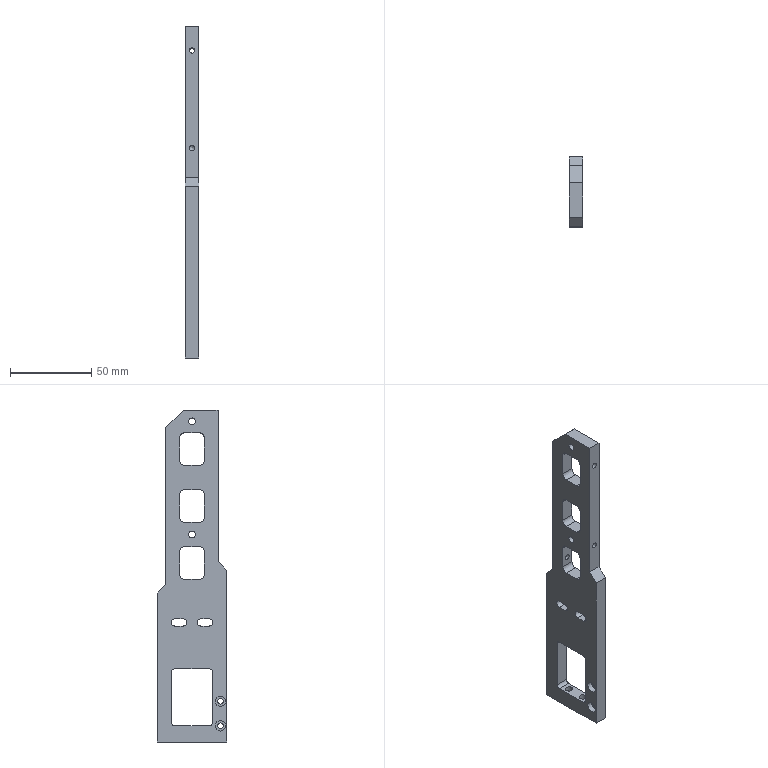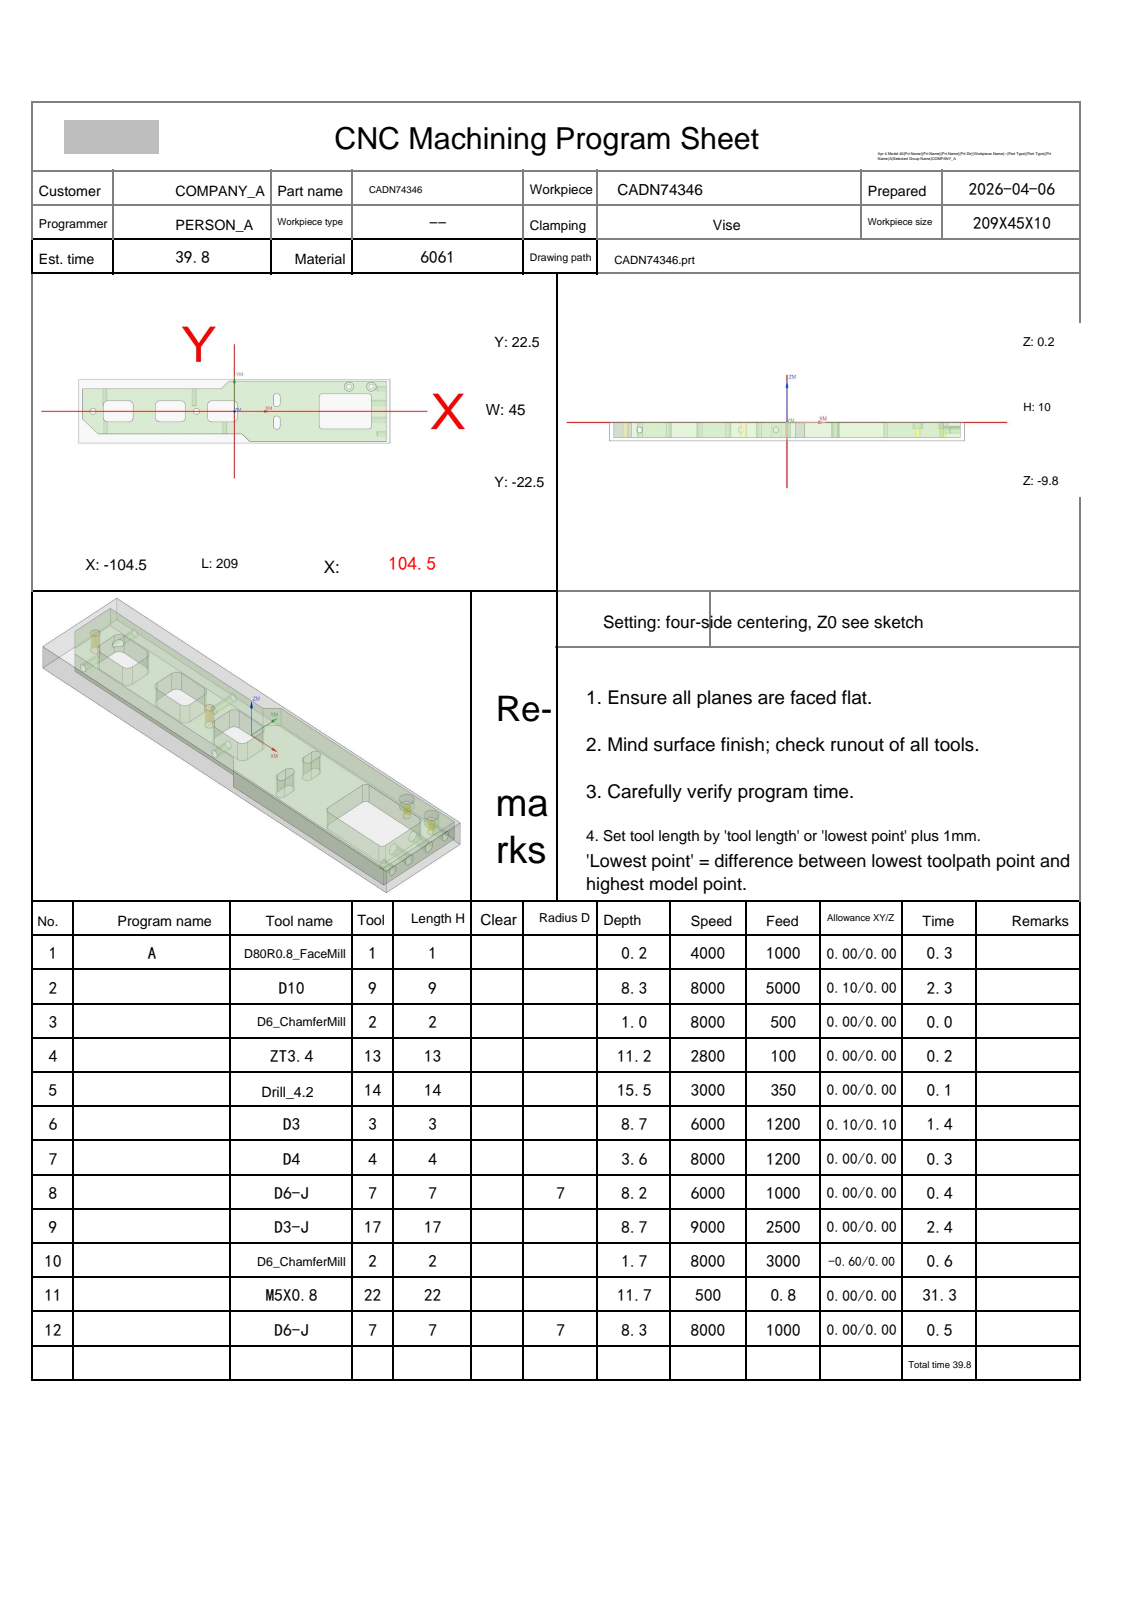NC program | NX | posted by the shop | part box 8 x 43 x 204 mm
Lines 1525 to 2600 of 14335:
N9 T17 M06
(D3-J  D=3. R=0. H=17 ce=0.00 di=0.01)
G00 G90 G54 X-70.087 Y2.104 M03 S6000
G43 H17 Z20.
M08
Z.154
G01 X-70.08 Z.085 F2000.
X-70.063 Y2.107 Z.024
X-70.035 Y2.111 Z-.031
X-70. Y2.117 Z-.08
X-69.957 Y2.126 Z-.123
X-69.909 Y2.136 Z-.16
X-69.858 Y2.15 Z-.192
X-69.804 Y2.166 Z-.219
X-69.75 Y2.185 Z-.242
X-69.697 Y2.208 Z-.26
X-69.647 Y2.234 Z-.274
X-69.6 Y2.263 Z-.284
X-69.559 Y2.296 Z-.291
X-69.525 Y2.333 Z-.295
X-69.5 Y2.375 Z-.296
Y4.5 F2500.
G03 X-71. Y6. I-1.5 J0.0
G01 X-73.125
X-73.154 Y5.984 Z-.297
X-73.159 Y5.939 Z-.3
X-73.143 Y5.867 Z-.304
X-73.107 Y5.772 Z-.31
X-73.052 Y5.657 Z-.316
X-72.982 Y5.525 Z-.324
X-72.801 Y5.228 Z-.343
X-72.673 Y5.034 Z-.355
X-72.449 Y4.722 Z-.377
X-72.079 Y4.266 Z-.41
X-71.674 Y3.832 Z-.444
X-71.24 Y3.425 Z-.479
X-70.783 Y3.054 Z-.512
X-70.47 Y2.829 Z-.533
X-70.276 Y2.701 Z-.546
X-69.977 Y2.519 Z-.565
X-69.845 Y2.449 Z-.573
X-69.729 Y2.394 Z-.579
X-69.634 Y2.358 Z-.585
X-69.562 Y2.341 Z-.589
X-69.516 Y2.346 Z-.592
X-69.5 Y2.375 Z-.593
Y4.5
G03 X-71. Y6. I-1.5 J0.0
G01 X-73.125
X-73.154 Y5.984
X-73.159 Y5.939 Z-.596
X-73.143 Y5.867 Z-.6
X-73.107 Y5.772 Z-.606
X-73.052 Y5.657 Z-.613
X-72.982 Y5.525 Z-.621
X-72.801 Y5.228 Z-.639
X-72.673 Y5.034 Z-.652
X-72.449 Y4.722 Z-.673
X-72.079 Y4.266 Z-.706
X-71.674 Y3.832 Z-.741
X-71.24 Y3.425 Z-.775
X-70.783 Y3.054 Z-.809
X-70.47 Y2.829 Z-.83
X-70.276 Y2.701 Z-.842
X-69.977 Y2.519 Z-.861
X-69.845 Y2.449 Z-.869
X-69.729 Y2.394 Z-.876
X-69.634 Y2.358 Z-.881
X-69.562 Y2.341 Z-.885
X-69.516 Y2.346 Z-.888
X-69.5 Y2.375 Z-.889
Y4.5
G03 X-71. Y6. I-1.5 J0.0
G01 X-73.125
X-73.154 Y5.984 Z-.89
X-73.159 Y5.939 Z-.892
X-73.143 Y5.867 Z-.897
X-73.107 Y5.772 Z-.902
X-73.052 Y5.657 Z-.909
X-72.982 Y5.525 Z-.917
X-72.801 Y5.228 Z-.936
X-72.673 Y5.034 Z-.948
X-72.449 Y4.722 Z-.969
X-72.079 Y4.266 Z-1.003
X-71.674 Y3.832 Z-1.037
X-71.24 Y3.425 Z-1.072
X-70.783 Y3.054 Z-1.105
X-70.47 Y2.829 Z-1.126
X-70.276 Y2.701 Z-1.139
X-69.977 Y2.519 Z-1.157
X-69.845 Y2.449 Z-1.165
X-69.729 Y2.394 Z-1.172
X-69.634 Y2.358 Z-1.178
X-69.562 Y2.341 Z-1.182
X-69.516 Y2.346 Z-1.184
X-69.5 Y2.375 Z-1.185
Y4.5
G03 X-71. Y6. I-1.5 J0.0
G01 X-73.125
X-73.154 Y5.984 Z-1.186
X-73.159 Y5.939 Z-1.189
X-73.143 Y5.867 Z-1.193
X-73.107 Y5.772 Z-1.198
X-73.052 Y5.657 Z-1.205
X-72.982 Y5.525 Z-1.213
X-72.801 Y5.228 Z-1.232
X-72.673 Y5.034 Z-1.244
X-72.449 Y4.722 Z-1.265
X-72.079 Y4.266 Z-1.299
X-71.674 Y3.832 Z-1.333
X-71.24 Y3.425 Z-1.368
X-70.783 Y3.054 Z-1.401
X-70.47 Y2.829 Z-1.422
X-70.276 Y2.701 Z-1.435
X-69.977 Y2.519 Z-1.453
X-69.845 Y2.449 Z-1.461
X-69.729 Y2.394 Z-1.468
X-69.634 Y2.358 Z-1.474
X-69.562 Y2.341 Z-1.478
X-69.516 Y2.346 Z-1.481
X-69.5 Y2.375
Y4.5
G03 X-71. Y6. I-1.5 J0.0
G01 X-73.125
X-73.154 Y5.984 Z-1.482
X-73.159 Y5.939 Z-1.485
X-73.143 Y5.867 Z-1.489
X-73.107 Y5.772 Z-1.495
X-73.052 Y5.657 Z-1.502
X-72.982 Y5.525 Z-1.51
X-72.801 Y5.228 Z-1.528
X-72.673 Y5.034 Z-1.541
X-72.449 Y4.722 Z-1.562
X-72.079 Y4.266 Z-1.595
X-71.674 Y3.832 Z-1.63
X-71.24 Y3.425 Z-1.664
X-70.783 Y3.054 Z-1.698
X-70.47 Y2.829 Z-1.719
X-70.276 Y2.701 Z-1.731
X-69.977 Y2.519 Z-1.75
X-69.845 Y2.449 Z-1.758
X-69.729 Y2.394 Z-1.765
X-69.634 Y2.358 Z-1.77
X-69.562 Y2.341 Z-1.774
X-69.516 Y2.346 Z-1.777
X-69.5 Y2.375 Z-1.778
Y4.5
G03 X-71. Y6. I-1.5 J0.0
G01 X-73.125
X-73.154 Y5.984 Z-1.779
X-73.159 Y5.939 Z-1.781
X-73.143 Y5.867 Z-1.785
X-73.107 Y5.772 Z-1.791
X-73.052 Y5.657 Z-1.798
X-72.982 Y5.525 Z-1.806
X-72.801 Y5.228 Z-1.824
X-72.673 Y5.034 Z-1.837
X-72.449 Y4.722 Z-1.858
X-72.079 Y4.266 Z-1.891
X-71.674 Y3.832 Z-1.926
X-71.24 Y3.425 Z-1.96
X-70.783 Y3.054 Z-1.994
X-70.47 Y2.829 Z-2.015
X-70.276 Y2.701 Z-2.027
X-69.977 Y2.519 Z-2.046
X-69.845 Y2.449 Z-2.054
X-69.729 Y2.394 Z-2.061
X-69.634 Y2.358 Z-2.066
X-69.562 Y2.341 Z-2.071
X-69.516 Y2.346 Z-2.073
X-69.5 Y2.375 Z-2.074
Y4.5
G03 X-71. Y6. I-1.5 J0.0
G01 X-73.125
X-73.154 Y5.984 Z-2.075
X-73.159 Y5.939 Z-2.078
X-73.143 Y5.867 Z-2.082
X-73.107 Y5.772 Z-2.087
X-73.052 Y5.657 Z-2.094
X-72.982 Y5.525 Z-2.102
X-72.801 Y5.228 Z-2.121
X-72.673 Y5.034 Z-2.133
X-72.449 Y4.722 Z-2.154
X-72.079 Y4.266 Z-2.188
X-71.674 Y3.832 Z-2.222
X-71.24 Y3.425 Z-2.257
X-70.783 Y3.054 Z-2.29
X-70.47 Y2.829 Z-2.311
X-70.276 Y2.701 Z-2.324
X-69.977 Y2.519 Z-2.342
X-69.845 Y2.449 Z-2.35
X-69.729 Y2.394 Z-2.357
X-69.634 Y2.358 Z-2.363
X-69.562 Y2.341 Z-2.367
X-69.516 Y2.346 Z-2.369
X-69.5 Y2.375 Z-2.37
Y4.5
G03 X-71. Y6. I-1.5 J0.0
G01 X-73.125
X-73.154 Y5.984 Z-2.371
X-73.159 Y5.939 Z-2.374
X-73.143 Y5.867 Z-2.378
X-73.107 Y5.772 Z-2.384
X-73.052 Y5.657 Z-2.39
X-72.982 Y5.525 Z-2.398
X-72.801 Y5.228 Z-2.417
X-72.673 Y5.034 Z-2.43
X-72.449 Y4.722 Z-2.451
X-72.079 Y4.266 Z-2.484
X-71.674 Y3.832 Z-2.519
X-71.24 Y3.425 Z-2.553
X-70.783 Y3.054 Z-2.586
X-70.47 Y2.829 Z-2.608
X-70.276 Y2.701 Z-2.62
X-69.977 Y2.519 Z-2.639
X-69.845 Y2.449 Z-2.647
X-69.729 Y2.394 Z-2.653
X-69.634 Y2.358 Z-2.659
X-69.562 Y2.341 Z-2.663
X-69.516 Y2.346 Z-2.666
X-69.5 Y2.375 Z-2.667
Y4.5
G03 X-71. Y6. I-1.5 J0.0
G01 X-73.125
X-73.154 Y5.984 Z-2.668
X-73.159 Y5.939 Z-2.67
X-73.143 Y5.867 Z-2.674
X-73.107 Y5.772 Z-2.68
X-73.052 Y5.657 Z-2.687
X-72.982 Y5.525 Z-2.695
X-72.801 Y5.228 Z-2.713
X-72.673 Y5.034 Z-2.726
X-72.449 Y4.722 Z-2.747
X-72.079 Y4.266 Z-2.78
X-71.674 Y3.832 Z-2.815
X-71.24 Y3.425 Z-2.849
X-70.783 Y3.054 Z-2.883
X-70.47 Y2.829 Z-2.904
X-70.276 Y2.701 Z-2.916
X-69.977 Y2.519 Z-2.935
X-69.845 Y2.449 Z-2.943
X-69.729 Y2.394 Z-2.95
X-69.634 Y2.358 Z-2.955
X-69.562 Y2.341 Z-2.959
X-69.516 Y2.346 Z-2.962
X-69.5 Y2.375 Z-2.963
Y4.5
G03 X-71. Y6. I-1.5 J0.0
G01 X-73.125
X-73.154 Y5.984 Z-2.964
X-73.159 Y5.939 Z-2.966
X-73.143 Y5.867 Z-2.971
X-73.107 Y5.772 Z-2.976
X-73.052 Y5.657 Z-2.983
X-72.982 Y5.525 Z-2.991
X-72.801 Y5.228 Z-3.01
X-72.673 Y5.034 Z-3.022
X-72.449 Y4.722 Z-3.043
X-72.079 Y4.266 Z-3.077
X-71.674 Y3.832 Z-3.111
X-71.24 Y3.425 Z-3.146
X-70.783 Y3.054 Z-3.179
X-70.47 Y2.829 Z-3.2
X-70.276 Y2.701 Z-3.213
X-69.977 Y2.519 Z-3.231
X-69.845 Y2.449 Z-3.239
X-69.729 Y2.394 Z-3.246
X-69.634 Y2.358 Z-3.252
X-69.562 Y2.341 Z-3.256
X-69.516 Y2.346 Z-3.258
X-69.5 Y2.375 Z-3.259
Y4.5
G03 X-71. Y6. I-1.5 J0.0
G01 X-73.125
X-73.154 Y5.984 Z-3.26
X-73.159 Y5.939 Z-3.263
X-73.143 Y5.867 Z-3.267
X-73.107 Y5.772 Z-3.272
X-73.052 Y5.657 Z-3.279
X-72.982 Y5.525 Z-3.287
X-72.801 Y5.228 Z-3.306
X-72.673 Y5.034 Z-3.318
X-72.449 Y4.722 Z-3.34
X-72.079 Y4.266 Z-3.373
X-71.674 Y3.832 Z-3.407
X-71.24 Y3.425 Z-3.442
X-70.783 Y3.054 Z-3.475
X-70.47 Y2.829 Z-3.496
X-70.276 Y2.701 Z-3.509
X-69.977 Y2.519 Z-3.528
X-69.845 Y2.449 Z-3.535
X-69.729 Y2.394 Z-3.542
X-69.634 Y2.358 Z-3.548
X-69.562 Y2.341 Z-3.552
X-69.516 Y2.346 Z-3.555
X-69.5 Y2.375 Z-3.556
Y4.5
G03 X-71. Y6. I-1.5 J0.0
G01 X-73.125
X-73.154 Y5.984
X-73.159 Y5.939 Z-3.559
X-73.143 Y5.867 Z-3.563
X-73.107 Y5.772 Z-3.569
X-73.052 Y5.657 Z-3.576
X-72.982 Y5.525 Z-3.584
X-72.801 Y5.228 Z-3.602
X-72.673 Y5.034 Z-3.615
X-72.449 Y4.722 Z-3.636
X-72.079 Y4.266 Z-3.669
X-71.674 Y3.832 Z-3.704
X-71.24 Y3.425 Z-3.738
X-70.783 Y3.054 Z-3.772
X-70.47 Y2.829 Z-3.793
X-70.276 Y2.701 Z-3.805
X-69.977 Y2.519 Z-3.824
X-69.845 Y2.449 Z-3.832
X-69.729 Y2.394 Z-3.839
X-69.634 Y2.358 Z-3.844
X-69.562 Y2.341 Z-3.848
X-69.516 Y2.346 Z-3.851
X-69.5 Y2.375 Z-3.852
Y4.5
G03 X-71. Y6. I-1.5 J0.0
G01 X-73.125
X-73.154 Y5.984 Z-3.853
X-73.159 Y5.939 Z-3.855
X-73.143 Y5.867 Z-3.859
X-73.107 Y5.772 Z-3.865
X-73.052 Y5.657 Z-3.872
X-72.982 Y5.525 Z-3.88
X-72.801 Y5.228 Z-3.899
X-72.673 Y5.034 Z-3.911
X-72.449 Y4.722 Z-3.932
X-72.079 Y4.266 Z-3.965
X-71.674 Y3.832 Z-4.
X-71.24 Y3.425 Z-4.035
X-70.783 Y3.054 Z-4.068
X-70.47 Y2.829 Z-4.089
X-70.276 Y2.701 Z-4.101
X-69.977 Y2.519 Z-4.12
X-69.845 Y2.449 Z-4.128
X-69.729 Y2.394 Z-4.135
X-69.634 Y2.358 Z-4.141
X-69.562 Y2.341 Z-4.145
X-69.516 Y2.346 Z-4.147
X-69.5 Y2.375 Z-4.148
Y4.5
G03 X-71. Y6. I-1.5 J0.0
G01 X-73.125
X-73.154 Y5.984 Z-4.149
X-73.159 Y5.939 Z-4.152
X-73.143 Y5.867 Z-4.156
X-73.107 Y5.772 Z-4.161
X-73.052 Y5.657 Z-4.168
X-72.982 Y5.525 Z-4.176
X-72.801 Y5.228 Z-4.195
X-72.673 Y5.034 Z-4.207
X-72.449 Y4.722 Z-4.228
X-72.079 Y4.266 Z-4.262
X-71.674 Y3.832 Z-4.296
X-71.24 Y3.425 Z-4.331
X-70.783 Y3.054 Z-4.364
X-70.47 Y2.829 Z-4.385
X-70.276 Y2.701 Z-4.398
X-69.977 Y2.519 Z-4.416
X-69.845 Y2.449 Z-4.424
X-69.729 Y2.394 Z-4.431
X-69.634 Y2.358 Z-4.437
X-69.562 Y2.341 Z-4.441
X-69.516 Y2.346 Z-4.444
X-69.5 Y2.375
Y4.5
G03 X-71. Y6. I-1.5 J0.0
G01 X-73.125
X-73.154 Y5.984 Z-4.445
X-73.159 Y5.939 Z-4.448
X-73.143 Y5.867 Z-4.452
X-73.107 Y5.772 Z-4.458
X-73.052 Y5.657 Z-4.465
X-72.982 Y5.525 Z-4.472
X-72.801 Y5.228 Z-4.491
X-72.673 Y5.034 Z-4.504
X-72.449 Y4.722 Z-4.525
X-72.079 Y4.266 Z-4.558
X-71.674 Y3.832 Z-4.593
X-71.24 Y3.425 Z-4.627
X-70.783 Y3.054 Z-4.66
X-70.47 Y2.829 Z-4.682
X-70.276 Y2.701 Z-4.694
X-69.977 Y2.519 Z-4.713
X-69.845 Y2.449 Z-4.721
X-69.729 Y2.394 Z-4.728
X-69.634 Y2.358 Z-4.733
X-69.562 Y2.341 Z-4.737
X-69.516 Y2.346 Z-4.74
X-69.5 Y2.375 Z-4.741
Y4.5
G03 X-71. Y6. I-1.5 J0.0
G01 X-73.125
X-73.154 Y5.984 Z-4.742
X-73.159 Y5.939 Z-4.744
X-73.143 Y5.867 Z-4.748
X-73.107 Y5.772 Z-4.754
X-73.052 Y5.657 Z-4.761
X-72.982 Y5.525 Z-4.769
X-72.801 Y5.228 Z-4.787
X-72.673 Y5.034 Z-4.8
X-72.449 Y4.722 Z-4.821
X-72.079 Y4.266 Z-4.854
X-71.674 Y3.832 Z-4.889
X-71.24 Y3.425 Z-4.923
X-70.783 Y3.054 Z-4.957
X-70.47 Y2.829 Z-4.978
X-70.276 Y2.701 Z-4.99
X-69.977 Y2.519 Z-5.009
X-69.845 Y2.449 Z-5.017
X-69.729 Y2.394 Z-5.024
X-69.634 Y2.358 Z-5.029
X-69.562 Y2.341 Z-5.034
X-69.516 Y2.346 Z-5.036
X-69.5 Y2.375 Z-5.037
Y4.5
G03 X-71. Y6. I-1.5 J0.0
G01 X-73.125
X-73.154 Y5.984 Z-5.038
X-73.159 Y5.939 Z-5.041
X-73.143 Y5.867 Z-5.045
X-73.107 Y5.772 Z-5.05
X-73.052 Y5.657 Z-5.057
X-72.982 Y5.525 Z-5.065
X-72.801 Y5.228 Z-5.084
X-72.673 Y5.034 Z-5.096
X-72.449 Y4.722 Z-5.117
X-72.079 Y4.266 Z-5.151
X-71.674 Y3.832 Z-5.185
X-71.24 Y3.425 Z-5.22
X-70.783 Y3.054 Z-5.253
X-70.47 Y2.829 Z-5.274
X-70.276 Y2.701 Z-5.287
X-69.977 Y2.519 Z-5.305
X-69.845 Y2.449 Z-5.313
X-69.729 Y2.394 Z-5.32
X-69.634 Y2.358 Z-5.326
X-69.562 Y2.341 Z-5.33
X-69.516 Y2.346 Z-5.332
X-69.5 Y2.375 Z-5.333
Y4.5
G03 X-71. Y6. I-1.5 J0.0
G01 X-73.125
X-73.154 Y5.984 Z-5.334
X-73.159 Y5.939 Z-5.337
X-73.143 Y5.867 Z-5.341
X-73.107 Y5.772 Z-5.347
X-73.052 Y5.657 Z-5.353
X-72.982 Y5.525 Z-5.361
X-72.801 Y5.228 Z-5.38
X-72.673 Y5.034 Z-5.392
X-72.449 Y4.722 Z-5.414
X-72.079 Y4.266 Z-5.447
X-71.674 Y3.832 Z-5.481
X-71.24 Y3.425 Z-5.516
X-70.783 Y3.054 Z-5.549
X-70.47 Y2.829 Z-5.57
X-70.276 Y2.701 Z-5.583
X-69.977 Y2.519 Z-5.602
X-69.845 Y2.449 Z-5.61
X-69.729 Y2.394 Z-5.616
X-69.634 Y2.358 Z-5.622
X-69.562 Y2.341 Z-5.626
X-69.516 Y2.346 Z-5.629
X-69.5 Y2.375 Z-5.63
Y4.5
G03 X-71. Y6. I-1.5 J0.0
G01 X-73.125
X-73.154 Y5.984 Z-5.631
X-73.159 Y5.939 Z-5.633
X-73.143 Y5.867 Z-5.637
X-73.107 Y5.772 Z-5.643
X-73.052 Y5.657 Z-5.65
X-72.982 Y5.525 Z-5.658
X-72.801 Y5.228 Z-5.676
X-72.673 Y5.034 Z-5.689
X-72.449 Y4.722 Z-5.71
X-72.079 Y4.266 Z-5.743
X-71.674 Y3.832 Z-5.778
X-71.24 Y3.425 Z-5.812
X-70.783 Y3.054 Z-5.846
X-70.47 Y2.829 Z-5.867
X-70.276 Y2.701 Z-5.879
X-69.977 Y2.519 Z-5.898
X-69.845 Y2.449 Z-5.906
X-69.729 Y2.394 Z-5.913
X-69.634 Y2.358 Z-5.918
X-69.562 Y2.341 Z-5.922
X-69.516 Y2.346 Z-5.925
X-69.5 Y2.375 Z-5.926
Y4.5
G03 X-71. Y6. I-1.5 J0.0
G01 X-73.125
X-73.154 Y5.984 Z-5.927
X-73.159 Y5.939 Z-5.929
X-73.143 Y5.867 Z-5.934
X-73.107 Y5.772 Z-5.939
X-73.052 Y5.657 Z-5.946
X-72.982 Y5.525 Z-5.954
X-72.801 Y5.228 Z-5.973
X-72.673 Y5.034 Z-5.985
X-72.449 Y4.722 Z-6.006
X-72.079 Y4.266 Z-6.04
X-71.674 Y3.832 Z-6.074
X-71.24 Y3.425 Z-6.109
X-70.783 Y3.054 Z-6.142
X-70.47 Y2.829 Z-6.163
X-70.276 Y2.701 Z-6.176
X-69.977 Y2.519 Z-6.194
X-69.845 Y2.449 Z-6.202
X-69.729 Y2.394 Z-6.209
X-69.634 Y2.358 Z-6.215
X-69.562 Y2.341 Z-6.219
X-69.516 Y2.346 Z-6.221
X-69.5 Y2.375 Z-6.222
Y4.5
G03 X-71. Y6. I-1.5 J0.0
G01 X-73.125
X-73.154 Y5.984 Z-6.223
X-73.159 Y5.939 Z-6.226
X-73.143 Y5.867 Z-6.23
X-73.107 Y5.772 Z-6.235
X-73.052 Y5.657 Z-6.242
X-72.982 Y5.525 Z-6.25
X-72.801 Y5.228 Z-6.269
X-72.673 Y5.034 Z-6.281
X-72.449 Y4.722 Z-6.302
X-72.079 Y4.266 Z-6.336
X-71.674 Y3.832 Z-6.37
X-71.24 Y3.425 Z-6.405
X-70.783 Y3.054 Z-6.438
X-70.47 Y2.829 Z-6.459
X-70.276 Y2.701 Z-6.472
X-69.977 Y2.519 Z-6.49
X-69.845 Y2.449 Z-6.498
X-69.729 Y2.394 Z-6.505
X-69.634 Y2.358 Z-6.511
X-69.562 Y2.341 Z-6.515
X-69.516 Y2.346 Z-6.518
X-69.5 Y2.375 Z-6.519
Y4.5
G03 X-71. Y6. I-1.5 J0.0
G01 X-73.125
X-73.154 Y5.984
X-73.159 Y5.939 Z-6.522
X-73.143 Y5.867 Z-6.526
X-73.107 Y5.772 Z-6.532
X-73.052 Y5.657 Z-6.539
X-72.982 Y5.525 Z-6.547
X-72.801 Y5.228 Z-6.565
X-72.673 Y5.034 Z-6.578
X-72.449 Y4.722 Z-6.599
X-72.079 Y4.266 Z-6.632
X-71.674 Y3.832 Z-6.667
X-71.24 Y3.425 Z-6.701
X-70.783 Y3.054 Z-6.735
X-70.47 Y2.829 Z-6.756
X-70.276 Y2.701 Z-6.768
X-69.977 Y2.519 Z-6.787
X-69.845 Y2.449 Z-6.795
X-69.729 Y2.394 Z-6.802
X-69.634 Y2.358 Z-6.807
X-69.562 Y2.341 Z-6.811
X-69.516 Y2.346 Z-6.814
X-69.5 Y2.375 Z-6.815
Y4.5
G03 X-71. Y6. I-1.5 J0.0
G01 X-73.125
X-73.154 Y5.984 Z-6.816
X-73.159 Y5.939 Z-6.818
X-73.143 Y5.867 Z-6.822
X-73.107 Y5.772 Z-6.828
X-73.052 Y5.657 Z-6.835
X-72.982 Y5.525 Z-6.843
X-72.801 Y5.228 Z-6.861
X-72.673 Y5.034 Z-6.874
X-72.449 Y4.722 Z-6.895
X-72.079 Y4.266 Z-6.928
X-71.674 Y3.832 Z-6.963
X-71.24 Y3.425 Z-6.997
X-70.783 Y3.054 Z-7.031
X-70.47 Y2.829 Z-7.052
X-70.276 Y2.701 Z-7.064
X-69.977 Y2.519 Z-7.083
X-69.845 Y2.449 Z-7.091
X-69.729 Y2.394 Z-7.098
X-69.634 Y2.358 Z-7.103
X-69.562 Y2.341 Z-7.108
X-69.516 Y2.346 Z-7.11
X-69.5 Y2.375 Z-7.111
Y4.5
G03 X-71. Y6. I-1.5 J0.0
G01 X-73.125
X-73.154 Y5.984 Z-7.112
X-73.159 Y5.939 Z-7.115
X-73.143 Y5.867 Z-7.119
X-73.107 Y5.772 Z-7.124
X-73.052 Y5.657 Z-7.131
X-72.982 Y5.525 Z-7.139
X-72.801 Y5.228 Z-7.158
X-72.673 Y5.034 Z-7.17
X-72.449 Y4.722 Z-7.191
X-72.079 Y4.266 Z-7.225
X-71.674 Y3.832 Z-7.259
X-71.24 Y3.425 Z-7.294
X-70.783 Y3.054 Z-7.327
X-70.47 Y2.829 Z-7.348
X-70.276 Y2.701 Z-7.361
X-69.977 Y2.519 Z-7.379
X-69.845 Y2.449 Z-7.387
X-69.729 Y2.394 Z-7.394
X-69.634 Y2.358 Z-7.4
X-69.562 Y2.341 Z-7.404
X-69.516 Y2.346 Z-7.407
X-69.5 Y2.375
Y4.5
G03 X-71. Y6. I-1.5 J0.0
G01 X-73.125
X-73.154 Y5.984 Z-7.408
X-73.159 Y5.939 Z-7.411
X-73.143 Y5.867 Z-7.415
X-73.107 Y5.772 Z-7.421
X-73.052 Y5.657 Z-7.427
X-72.982 Y5.525 Z-7.435
X-72.801 Y5.228 Z-7.454
X-72.673 Y5.034 Z-7.467
X-72.449 Y4.722 Z-7.488
X-72.079 Y4.266 Z-7.521
X-71.674 Y3.832 Z-7.556
X-71.24 Y3.425 Z-7.59
X-70.783 Y3.054 Z-7.623
X-70.47 Y2.829 Z-7.645
X-70.276 Y2.701 Z-7.657
X-69.977 Y2.519 Z-7.676
X-69.845 Y2.449 Z-7.684
X-69.729 Y2.394 Z-7.69
X-69.634 Y2.358 Z-7.696
X-69.562 Y2.341 Z-7.7
X-69.516 Y2.346 Z-7.703
X-69.5 Y2.375 Z-7.704
Y4.5
G03 X-71. Y6. I-1.5 J0.0
G01 X-73.125
X-73.154 Y5.984 Z-7.705
X-73.159 Y5.939 Z-7.707
X-73.143 Y5.867 Z-7.711
X-73.107 Y5.772 Z-7.717
X-73.052 Y5.657 Z-7.724
X-72.982 Y5.525 Z-7.732
X-72.801 Y5.228 Z-7.75
X-72.673 Y5.034 Z-7.763
X-72.449 Y4.722 Z-7.784
X-72.079 Y4.266 Z-7.817
X-71.674 Y3.832 Z-7.852
X-71.24 Y3.425 Z-7.886
X-70.783 Y3.054 Z-7.92
X-70.47 Y2.829 Z-7.941
X-70.276 Y2.701 Z-7.953
X-69.977 Y2.519 Z-7.972
X-69.845 Y2.449 Z-7.98
X-69.729 Y2.394 Z-7.987
X-69.634 Y2.358 Z-7.992
X-69.562 Y2.341 Z-7.997
X-69.516 Y2.346 Z-7.999
X-69.5 Y2.375 Z-8.
Y4.5
G03 X-71. Y6. I-1.5 J0.0
G01 X-73.125
X-73.167 Y5.975 Z-7.999
X-73.204 Y5.941 Z-7.995
X-73.237 Y5.901 Z-7.988
X-73.267 Y5.855 Z-7.977
X-73.292 Y5.805 Z-7.963
X-73.315 Y5.753 Z-7.945
X-73.334 Y5.7 Z-7.923
X-73.351 Y5.647 Z-7.896
X-73.364 Y5.597 Z-7.864
X-73.375 Y5.55 Z-7.827
X-73.384 Y5.509 Z-7.784
X-73.39 Y5.473 Z-7.735
X-73.394 Y5.447 Z-7.68
X-73.396 Y5.429 Z-7.618
X-73.397 Y5.423 Z-7.55
G00 Z3.
X-82.603
Z.154
G01 X-82.604 Y5.429 Z.085 F2000.
X-82.606 Y5.447 Z.024
X-82.61 Y5.473 Z-.031
X-82.616 Y5.509 Z-.08
X-82.625 Y5.55 Z-.123
X-82.636 Y5.597 Z-.16
X-82.649 Y5.647 Z-.192
X-82.666 Y5.7 Z-.219
X-82.685 Y5.753 Z-.242
X-82.708 Y5.805 Z-.26
X-82.733 Y5.855 Z-.274
X-82.763 Y5.901 Z-.284
X-82.796 Y5.941 Z-.291
X-82.833 Y5.975 Z-.295
X-82.875 Y6. Z-.296
X-85. F2500.
G03 X-86.5 Y4.5 I0.0 J-1.5
G01 Y2.375
X-86.484 Y2.346 Z-.297
X-86.439 Y2.341 Z-.3
X-86.367 Y2.357 Z-.304
X-86.272 Y2.393 Z-.31
X-86.157 Y2.448 Z-.316
X-86.025 Y2.518 Z-.324
X-85.727 Y2.699 Z-.343
X-85.534 Y2.827 Z-.355
X-85.221 Y3.051 Z-.377
X-84.765 Y3.422 Z-.41
X-84.331 Y3.829 Z-.444
X-83.924 Y4.263 Z-.479
X-83.553 Y4.72 Z-.512
X-83.329 Y5.033 Z-.533
X-83.2 Y5.227 Z-.546
X-83.019 Y5.524 Z-.565
X-82.948 Y5.657 Z-.573
X-82.894 Y5.772 Z-.579
X-82.858 Y5.867 Z-.585
X-82.841 Y5.939 Z-.589
X-82.846 Y5.984 Z-.592
X-82.875 Y6. Z-.593
X-85.
G03 X-86.5 Y4.5 I0.0 J-1.5
G01 Y2.375
X-86.484 Y2.346
X-86.439 Y2.341 Z-.596
X-86.367 Y2.357 Z-.6
X-86.272 Y2.393 Z-.606
X-86.157 Y2.448 Z-.613
X-86.025 Y2.518 Z-.621
X-85.727 Y2.699 Z-.639
X-85.534 Y2.827 Z-.652
X-85.221 Y3.051 Z-.673
X-84.765 Y3.422 Z-.706
X-84.331 Y3.829 Z-.741
X-83.924 Y4.263 Z-.775
X-83.553 Y4.72 Z-.809
X-83.329 Y5.033 Z-.83
X-83.2 Y5.227 Z-.842
X-83.019 Y5.524 Z-.861
X-82.948 Y5.657 Z-.869
X-82.894 Y5.772 Z-.876
X-82.858 Y5.867 Z-.881
X-82.841 Y5.939 Z-.885
X-82.846 Y5.984 Z-.888
X-82.875 Y6. Z-.889
X-85.
G03 X-86.5 Y4.5 I0.0 J-1.5
G01 Y2.375
X-86.484 Y2.346 Z-.89
X-86.439 Y2.341 Z-.892
X-86.367 Y2.357 Z-.897
X-86.272 Y2.393 Z-.902
X-86.157 Y2.448 Z-.909
X-86.025 Y2.518 Z-.917
X-85.727 Y2.699 Z-.936
X-85.534 Y2.827 Z-.948
X-85.221 Y3.051 Z-.969
X-84.765 Y3.422 Z-1.003
X-84.331 Y3.829 Z-1.037
X-83.924 Y4.263 Z-1.072
X-83.553 Y4.72 Z-1.105
X-83.329 Y5.033 Z-1.126
X-83.2 Y5.227 Z-1.139
X-83.019 Y5.524 Z-1.157
X-82.948 Y5.657 Z-1.165
X-82.894 Y5.772 Z-1.172
X-82.858 Y5.867 Z-1.178
X-82.841 Y5.939 Z-1.182
X-82.846 Y5.984 Z-1.184
X-82.875 Y6. Z-1.185
X-85.
G03 X-86.5 Y4.5 I0.0 J-1.5
G01 Y2.375
X-86.484 Y2.346 Z-1.186
X-86.439 Y2.341 Z-1.189
X-86.367 Y2.357 Z-1.193
X-86.272 Y2.393 Z-1.198
X-86.157 Y2.448 Z-1.205
X-86.025 Y2.518 Z-1.213
X-85.727 Y2.699 Z-1.232
X-85.534 Y2.827 Z-1.244
X-85.221 Y3.051 Z-1.265
X-84.765 Y3.422 Z-1.299
X-84.331 Y3.829 Z-1.333
X-83.924 Y4.263 Z-1.368
X-83.553 Y4.72 Z-1.401
X-83.329 Y5.033 Z-1.422
X-83.2 Y5.227 Z-1.435
X-83.019 Y5.524 Z-1.453
X-82.948 Y5.657 Z-1.461
X-82.894 Y5.772 Z-1.468
X-82.858 Y5.867 Z-1.474
X-82.841 Y5.939 Z-1.478
X-82.846 Y5.984 Z-1.481
X-82.875 Y6.
X-85.
G03 X-86.5 Y4.5 I0.0 J-1.5
G01 Y2.375
X-86.484 Y2.346 Z-1.482
X-86.439 Y2.341 Z-1.485
X-86.367 Y2.357 Z-1.489
X-86.272 Y2.393 Z-1.495
X-86.157 Y2.448 Z-1.502
X-86.025 Y2.518 Z-1.51
X-85.727 Y2.699 Z-1.528
X-85.534 Y2.827 Z-1.541
X-85.221 Y3.051 Z-1.562
X-84.765 Y3.422 Z-1.595
X-84.331 Y3.829 Z-1.63
X-83.924 Y4.263 Z-1.664
X-83.553 Y4.72 Z-1.698
X-83.329 Y5.033 Z-1.719
X-83.2 Y5.227 Z-1.731
X-83.019 Y5.524 Z-1.75
X-82.948 Y5.657 Z-1.758
X-82.894 Y5.772 Z-1.765
X-82.858 Y5.867 Z-1.77
X-82.841 Y5.939 Z-1.774
X-82.846 Y5.984 Z-1.777
X-82.875 Y6. Z-1.778
X-85.
G03 X-86.5 Y4.5 I0.0 J-1.5
G01 Y2.375
X-86.484 Y2.346 Z-1.779
X-86.439 Y2.341 Z-1.781
X-86.367 Y2.357 Z-1.785
X-86.272 Y2.393 Z-1.791
X-86.157 Y2.448 Z-1.798
X-86.025 Y2.518 Z-1.806
X-85.727 Y2.699 Z-1.824
X-85.534 Y2.827 Z-1.837
X-85.221 Y3.051 Z-1.858
X-84.765 Y3.422 Z-1.891
X-84.331 Y3.829 Z-1.926
X-83.924 Y4.263 Z-1.96
X-83.553 Y4.72 Z-1.994
X-83.329 Y5.033 Z-2.015
X-83.2 Y5.227 Z-2.027
X-83.019 Y5.524 Z-2.046
X-82.948 Y5.657 Z-2.054
X-82.894 Y5.772 Z-2.061
X-82.858 Y5.867 Z-2.066
X-82.841 Y5.939 Z-2.071
X-82.846 Y5.984 Z-2.073
X-82.875 Y6. Z-2.074
X-85.
G03 X-86.5 Y4.5 I0.0 J-1.5
G01 Y2.375
X-86.484 Y2.346 Z-2.075
X-86.439 Y2.341 Z-2.078
X-86.367 Y2.357 Z-2.082
X-86.272 Y2.393 Z-2.087
X-86.157 Y2.448 Z-2.094
X-86.025 Y2.518 Z-2.102
X-85.727 Y2.699 Z-2.121
X-85.534 Y2.827 Z-2.133
X-85.221 Y3.051 Z-2.154
X-84.765 Y3.422 Z-2.188
X-84.331 Y3.829 Z-2.222
X-83.924 Y4.263 Z-2.257
X-83.553 Y4.72 Z-2.29
X-83.329 Y5.033 Z-2.311
X-83.2 Y5.227 Z-2.324
X-83.019 Y5.524 Z-2.342
X-82.948 Y5.657 Z-2.35
X-82.894 Y5.772 Z-2.357
X-82.858 Y5.867 Z-2.363
X-82.841 Y5.939 Z-2.367
X-82.846 Y5.984 Z-2.369
X-82.875 Y6. Z-2.37
X-85.
G03 X-86.5 Y4.5 I0.0 J-1.5
G01 Y2.375
X-86.484 Y2.346 Z-2.371
X-86.439 Y2.341 Z-2.374
X-86.367 Y2.357 Z-2.378
X-86.272 Y2.393 Z-2.384
X-86.157 Y2.448 Z-2.39
X-86.025 Y2.518 Z-2.398
X-85.727 Y2.699 Z-2.417
X-85.534 Y2.827 Z-2.43
X-85.221 Y3.051 Z-2.451
X-84.765 Y3.422 Z-2.484
X-84.331 Y3.829 Z-2.519
X-83.924 Y4.263 Z-2.553
X-83.553 Y4.72 Z-2.586
X-83.329 Y5.033 Z-2.608
X-83.2 Y5.227 Z-2.62
X-83.019 Y5.524 Z-2.639
X-82.948 Y5.657 Z-2.647
X-82.894 Y5.772 Z-2.653
X-82.858 Y5.867 Z-2.659
X-82.841 Y5.939 Z-2.663
X-82.846 Y5.984 Z-2.666
X-82.875 Y6. Z-2.667
X-85.
G03 X-86.5 Y4.5 I0.0 J-1.5
G01 Y2.375
X-86.484 Y2.346 Z-2.668
X-86.439 Y2.341 Z-2.67
X-86.367 Y2.357 Z-2.674
X-86.272 Y2.393 Z-2.68
X-86.157 Y2.448 Z-2.687
X-86.025 Y2.518 Z-2.695
X-85.727 Y2.699 Z-2.713
X-85.534 Y2.827 Z-2.726
X-85.221 Y3.051 Z-2.747
X-84.765 Y3.422 Z-2.78
X-84.331 Y3.829 Z-2.815
X-83.924 Y4.263 Z-2.849
X-83.553 Y4.72 Z-2.883
X-83.329 Y5.033 Z-2.904
X-83.2 Y5.227 Z-2.916
X-83.019 Y5.524 Z-2.935
X-82.948 Y5.657 Z-2.943
X-82.894 Y5.772 Z-2.95
X-82.858 Y5.867 Z-2.955
X-82.841 Y5.939 Z-2.959
X-82.846 Y5.984 Z-2.962
X-82.875 Y6. Z-2.963
X-85.
G03 X-86.5 Y4.5 I0.0 J-1.5
G01 Y2.375
X-86.484 Y2.346 Z-2.964
X-86.439 Y2.34 Z-2.966
X-86.367 Y2.355 Z-2.971
X-86.271 Y2.39 Z-2.976
X-86.156 Y2.443 Z-2.983
X-86.024 Y2.512 Z-2.991
X-85.793 Y2.647 Z-3.005
X-85.532 Y2.817 Z-3.022
X-85.218 Y3.039 Z-3.043
X-84.762 Y3.41 Z-3.077
X-84.328 Y3.817 Z-3.111
X-83.923 Y4.254 Z-3.146
X-83.552 Y4.713 Z-3.179
X-83.328 Y5.028 Z-3.2
X-83.2 Y5.223 Z-3.213
X-83.019 Y5.522 Z-3.231
X-82.948 Y5.655 Z-3.239
X-82.894 Y5.771 Z-3.246
X-82.857 Y5.866 Z-3.252
X-82.841 Y5.938 Z-3.256
X-82.846 Y5.984 Z-3.258
X-82.875 Y6. Z-3.259
X-85.
G03 X-86.5 Y4.5 I0.0 J-1.5
G01 Y2.375
X-86.484 Y2.346 Z-3.26
X-86.439 Y2.34 Z-3.263
X-86.367 Y2.355 Z-3.267
X-86.271 Y2.39 Z-3.272
X-86.156 Y2.443 Z-3.279
X-86.024 Y2.512 Z-3.287
X-85.793 Y2.647 Z-3.302
X-85.532 Y2.817 Z-3.318
X-85.218 Y3.039 Z-3.34
X-84.762 Y3.41 Z-3.373
X-84.328 Y3.817 Z-3.407
X-83.923 Y4.254 Z-3.442
X-83.552 Y4.713 Z-3.475
X-83.328 Y5.028 Z-3.496
X-83.2 Y5.223 Z-3.509
X-83.019 Y5.522 Z-3.528
X-82.948 Y5.655 Z-3.535
X-82.894 Y5.771 Z-3.542
X-82.857 Y5.866 Z-3.548
X-82.841 Y5.938 Z-3.552
X-82.846 Y5.984 Z-3.555
X-82.875 Y6. Z-3.556
X-85.
G03 X-86.5 Y4.5 I0.0 J-1.5
G01 Y2.375
X-86.484 Y2.346
X-86.439 Y2.34 Z-3.559
X-86.367 Y2.355 Z-3.563
X-86.271 Y2.39 Z-3.569
X-86.156 Y2.443 Z-3.576
X-86.024 Y2.512 Z-3.584
X-85.793 Y2.647 Z-3.598
X-85.532 Y2.817 Z-3.615
X-85.218 Y3.039 Z-3.636
X-84.762 Y3.41 Z-3.669
X-84.328 Y3.817 Z-3.704
X-83.923 Y4.254 Z-3.738
X-83.552 Y4.713 Z-3.772
X-83.328 Y5.028 Z-3.793
X-83.2 Y5.223 Z-3.805
X-83.019 Y5.522 Z-3.824
X-82.948 Y5.655 Z-3.832
X-82.894 Y5.771 Z-3.839
X-82.857 Y5.866 Z-3.844
X-82.841 Y5.938 Z-3.848
X-82.846 Y5.984 Z-3.851
X-82.875 Y6. Z-3.852
X-85.
G03 X-86.5 Y4.5 I0.0 J-1.5
G01 Y2.375
X-86.484 Y2.346 Z-3.853
X-86.439 Y2.34 Z-3.855
X-86.367 Y2.355 Z-3.859
X-86.271 Y2.39 Z-3.865
X-86.156 Y2.443 Z-3.872
X-86.024 Y2.512 Z-3.88
X-85.793 Y2.647 Z-3.894
X-85.532 Y2.817 Z-3.911
X-85.218 Y3.039 Z-3.932
X-84.762 Y3.41 Z-3.965
X-84.328 Y3.817 Z-4.
X-83.923 Y4.254 Z-4.035
X-83.552 Y4.713 Z-4.068
X-83.328 Y5.028 Z-4.089
X-83.2 Y5.223 Z-4.101
X-83.019 Y5.522 Z-4.12
X-82.948 Y5.655 Z-4.128
X-82.894 Y5.771 Z-4.135
X-82.857 Y5.866 Z-4.141
X-82.841 Y5.938 Z-4.145
X-82.846 Y5.984 Z-4.147
X-82.875 Y6. Z-4.148
X-85.
G03 X-86.5 Y4.5 I0.0 J-1.5
G01 Y2.375
X-86.484 Y2.346 Z-4.149
X-86.439 Y2.34 Z-4.152
X-86.367 Y2.355 Z-4.156
X-86.271 Y2.39 Z-4.161
X-86.156 Y2.443 Z-4.168
X-86.024 Y2.512 Z-4.176
X-85.793 Y2.647 Z-4.19
X-85.532 Y2.817 Z-4.207
X-85.218 Y3.039 Z-4.228
X-84.762 Y3.41 Z-4.262
X-84.328 Y3.817 Z-4.296
X-83.923 Y4.254 Z-4.331
X-83.552 Y4.713 Z-4.364
X-83.328 Y5.028 Z-4.385
X-83.2 Y5.223 Z-4.398
X-83.019 Y5.522 Z-4.416
X-82.948 Y5.655 Z-4.424
X-82.894 Y5.771 Z-4.431
X-82.857 Y5.866 Z-4.437
X-82.841 Y5.938 Z-4.441
X-82.846 Y5.984 Z-4.444
X-82.875 Y6.
X-85.
G03 X-86.484 Y4.718 I0.0 J-1.5
G01 X-86.485 Y4.694
X-86.495 Y4.627
X-86.5 Y4.5
Y2.375
X-86.484 Y2.346 Z-4.445
X-86.439 Y2.34 Z-4.448
X-86.367 Y2.355 Z-4.452
X-86.271 Y2.39 Z-4.458
X-86.156 Y2.443 Z-4.465
X-86.024 Y2.512 Z-4.472
X-85.793 Y2.647 Z-4.487
X-85.532 Y2.817 Z-4.504
X-85.218 Y3.039 Z-4.525
X-84.762 Y3.41 Z-4.558
X-84.328 Y3.817 Z-4.593
X-83.923 Y4.254 Z-4.627
X-83.552 Y4.713 Z-4.66